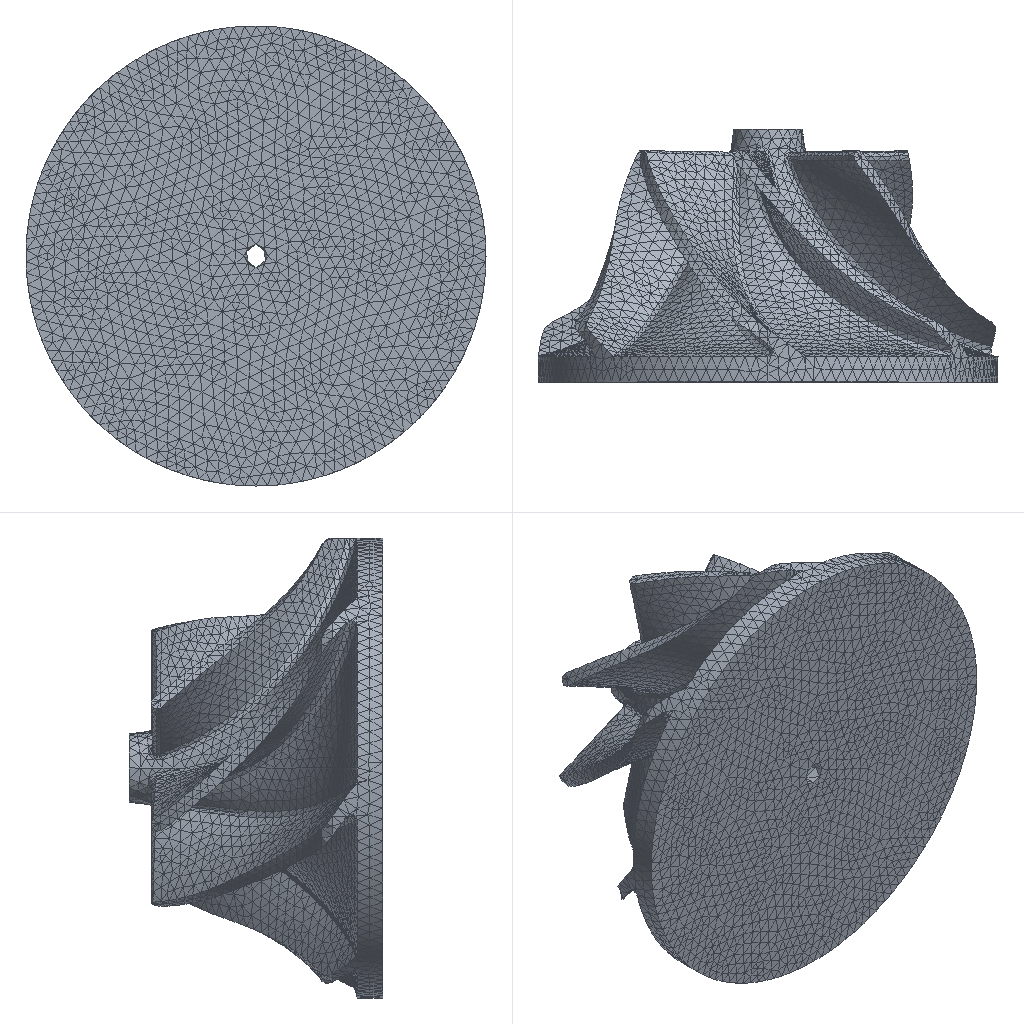Simulation study | ansys workbench
Set-up summary:
category,name,step,type,value,unit,region
solver,ansys_mapdl
solver,version,,,22.2
units,MPA,,stated
analysis,deck,,static,static
load_step,requested,,,1
analysis,nlgeom,,,True
mesh,nodes,,,125722
mesh,elements,,,83870
element_type,ANSYS 187 (type 1),,solid,83870
load,load commands in deck,,count,1
bc,support commands in deck,,count,3
named_set,CM_ROTVELCITY32,,component
named_set,_DISPZEROUX,,component
named_set,_DISPZEROUY,,component
named_set,_DISPZEROUZ,,component
material,1,,in results
check,setup vs results,,match
Ansys APDL input file, long lists of numbers shortened:
/batch
/config,noeldb,1     ! force off writing results to database
*get,_wallstrt,active,,time,wall
! ANSYS input file written by Workbench version 2022 R2
! File used for geometry attach: D:\虚拟C盘\仿\Centrifugal-impeller.STEP
/title,_____--____ (A5)
! ****** Begin Custom Load Command Snippet ******
/COM, ACT Extensions:
/COM,     LSDYNA, 2022.2
/COM,/COM,     ANSYSMotion, 2022.2
/COM,
! ****** End   Custom Load Command Snippet ******
*DIM,_wb_ProjectScratch_dir,string,248
_wb_ProjectScratch_dir(1) = 'F:\仿真模型\有限元\_ProjectScratch\Scr58A9\'
*DIM,_wb_SolverFiles_dir,string,248
_wb_SolverFiles_dir(1) = 'F:\仿真模型\有限元\叶轮带风扇_files\dp0\SYS\MECH\'
*DIM,_wb_userfiles_dir,string,248
_wb_userfiles_dir(1) = 'F:\仿真模型\有限元\叶轮带风扇_files\user_files\'
/com,--- Data in consistent NMM units. See Solving Units in the help system for more information.
/units,MPA
/nopr
/wb,file,start              !  signify a WB generated input file
/prep7
! Turn off shape checking because checks already performed inside WB mesher.
! See help system for more information.
SHPP,OFF,,NOWARN
/nolist
etcon,set             ! allow ANSYS to choose best KEYOP's for 180x elements, resets any applicable keyopt to MAPDL defaults
/com,*********** Nodes for the whole assembly ***********
nblock,3,,138294
(1i9,3e20.9e3)
        1    -1.900616311E-07     1.103362159E+01     1.000000000E+02
! (125721 more lines like these left out)
-1
/wb,elem,start            !  set before creation of elements
/com,*********** Elements for Body 1 "Centrifugal-impeller-FreeParts|__1" ***********
et,1,187
eblock,19,solid,,83870
(19i9)
        1        1        1        1        0        0        0        0       10        0        1     9101    17502    15417    16709    80423   124112    80419    80420
! (167739 more lines like these left out)
-1
/wb,elem,end               !  done creating elements
/com,*********** Send User Defined Coordinate System(s) ***********
csys,0
toffst,273.15,  ! Temperature offset from absolute zero
/com,*********** Set Reference Temperature ***********
tref,22.
/wb,mat,start              !  starting to send materials
/com,*********** Send Materials ***********
Temperature = 'TEMP' ! Temperature
MP,DENS,1,2.77e-09,	! tonne mm^-3
MP,ALPX,1,2.3e-05,	! C^-1
MP,C,1,875000000,	! mm^2 s^-2 C^-1
MPTEMP,,,,,,,,
MPTEMP,1,-100
MPTEMP,2,0
MPTEMP,3,100
MPTEMP,4,200
MPDATA,KXX,1, ,114,144,165,175,	! tonne mm s^-3 C^-1
MPTEMP,,,,,,,,
MPTEMP,,,,,,,,
MPTEMP,1,0
MPTEMP,2,20
MPTEMP,3,100
MPDATA,RSVX,1, ,2.43e-05,2.67e-05,3.63e-05,	! ohm mm
MPTEMP,,,,,,,,
MP,EX,1,75000,	! tonne s^-2 mm^-1
MP,NUXY,1,0.25,
MP,MURX,1,1,
/wb,mat,end                !  done sending materials
!************************* Model Summary ********************
!Centrifugal-impeller-FreeParts|__1,	铝合金,	matid,	1
!************************* End Model Summary ********************
! get the diagonal of the bounding box. Needed later for other things
*get,_xmin,node,,mnloc,x
*get,_ymin,node,,mnloc,y
*get,_zmin,node,,mnloc,z
*get,_xmax,node,,mxloc,x
*get,_ymax,node,,mxloc,y
*get,_zmax,node,,mxloc,z
_ASMDIAG=(_xmax-_xmin)*(_xmax-_xmin)+(_ymax-_ymin)*(_ymax-_ymin)+(_zmax-_zmin)*(_zmax-_zmin)
_ASMDIAG=SQRT(_ASMDIAG)
/wb,contact,start          !  starting to send contact
/wb,contact,end            !  done creating contacts
/golist
/wb,load,start             !  starting to send loads
/com,******* Constant Zero Displacement X *******
CMBLOCK,_DISPZEROUX,NODE,     5430
(8i10)
         6         9        10        11        12        13        14        15
! (678 more lines like these left out)
cmsel,s,_DISPZEROUX
d,all,ux,0
nsel,all
/com,******* Constant Zero Displacement Y *******
CMBLOCK,_DISPZEROUY,NODE,     5430
(8i10)
         6         9        10        11        12        13        14        15
! (678 more lines like these left out)
cmsel,s,_DISPZEROUY
d,all,uy,0
nsel,all
/com,******* Constant Zero Displacement Z *******
CMBLOCK,_DISPZEROUZ,NODE,     5430
(8i10)
         6         9        10        11        12        13        14        15
! (678 more lines like these left out)
cmsel,s,_DISPZEROUZ
d,all,uz,0
nsel,all
/com,*********** Define Rotational Velocity ***********
esel,none
esel,a,type,,1
cm,cm_rotvelcity32,elem
esel,all
/gst,on,on
fini
*get,_numnode,node,0,count
*get,_numelem,elem,0,count
*get, _MAXELEMNUM, elem, 0, NUM, MAX
*get, _MAXNODENUM, node, 0, NUM, MAX
*get, _MAXELEMTYPE, etyp, 0, NUM, MAX
*get, _MAXREALCONST, rcon, 0, NUM, MAX
/go
/wb,load,end               !  done creating loads
/com,--- Number of total nodes = %_numnode%
/com,--- Number of contact elements = 0
/com,--- Number of spring elements = 0
/com,--- Number of bearing elements = 0
/com,--- Number of solid elements = 83870
/com,--- Number of condensed parts = 0
/com,--- Number of total elements = %_numelem%
*get,_wallbsol,active,,time,wall
/com,****************************************************************************
/com,*************************    SOLUTION       ********************************
/com,****************************************************************************
/solu
antype,0                   ! static analysis
nlgeom,on                  ! Turn on Large Deformation Effects
_thickRatio=  1     ! Ratio of thick parts in the model
eqsl,pcg,1e-8,,,,,,1
cntr,print,1               ! print out contact info and also make no initial contact an error
dmpoption,emat,no             ! Don't combine emat file for DANSYS
dmpoption,esav,no             ! Don't combine esav file for DANSYS
nldiag,cont,iter           ! print out contact info each equilibrium iteration
rescontrol,define,last,last,,dele	   ! Program Controlled
/com,****************************************************
/com,******************* SOLVE FOR LS 1 OF 1 ****************
cmom,cm_rotvelcity32,0.,-2000.,0.,0.,55.,-5.
/nopr
/gopr
autots,on                  ! Workbench Program Controlled automatic time stepping
nsub,1,10,1                ! due to presence of general nonlinear
time,1.
outres,erase
outres,all,none
outres,nsol,all,
outres,rsol,all
outres,eangl,all
outres,etmp,all
outres,veng,all
outres,strs,all,
outres,epel,all,
outres,eppl,all,
outres,cont,all,
! *********** WB SOLVE COMMAND ***********
! check interactive state
*get,ANSINTER_,active,,int
*if,ANSINTER_,ne,0,then
/eof
*endif
solve
/com *************** Write FE CONNECTORS *********
CEWRITE,file,ce,,INTE
/com,****************************************************
/com,*************** FINISHED SOLVE FOR LS 1 *************
*get,_wallasol,active,,time,wall
/nopr
*get,_numnode,node,0,count
*get,_numelem,elem,0,count
*get, _MAXELEMNUM, elem, 0, NUM, MAX
*get, _MAXNODENUM, node, 0, NUM, MAX,,,INTERNAL
*get, _MAXELEMTYPE, etyp, 0, NUM, MAX
*get, _MAXREALCONST, rcon, 0, NUM, MAX
*get,_NSOLTHREADS,active,0,ntfs
*get,_NSOLPROCESSES,active,0,npfs
/gopr
*get,_PCGITER,active,,solu,cgiter
/post1
xmlo,ENCODING,ISO-8859-1
xmlo,parm
/xml,parm,xml
fini
/gopr
*get,_walldone,active,,time,wall
_preptime=(_wallbsol-_wallstrt)*3600
_solvtime=(_wallasol-_wallbsol)*3600
_posttime=(_walldone-_wallasol)*3600
_totaltim=(_walldone-_wallstrt)*3600
*get,_dlbratio,active,0,solu,dlbr
*get,_combtime,active,0,solu,comb
*get,_ssmode,active,0,solu,ssmm
*get,_ndofs,active,0,solu,ndof
*get,_sol_end_time,active,0,set,time
*if,_sol_end_time,eq,1.,then
/fclean				!clean distributed files
*endif
/com,--- Total number of nodes = %_numnode%
/com,--- Total number of elements = %_numelem%
/com,--- Element load balance ratio = %_dlbratio%
/com,--- Time to combine distributed files = %_combtime%
/com,--- Sparse memory mode = %_ssmode%
/com,--- Number of DOF = %_ndofs%
/wb,file,end               ! done with WB generated input
Results summary:
result,analysis,,,static
result,last_loadstep,,,1
result,primary field,,,displacement
result,reaction total,1,FX,0.4249,N
result,reaction total,1,FY,-0.000259,N
result,reaction total,1,FZ,-61490.78,N
result,mass,,,0.003073,"NMM: mm, ton, N, s, mV, mA, degC"